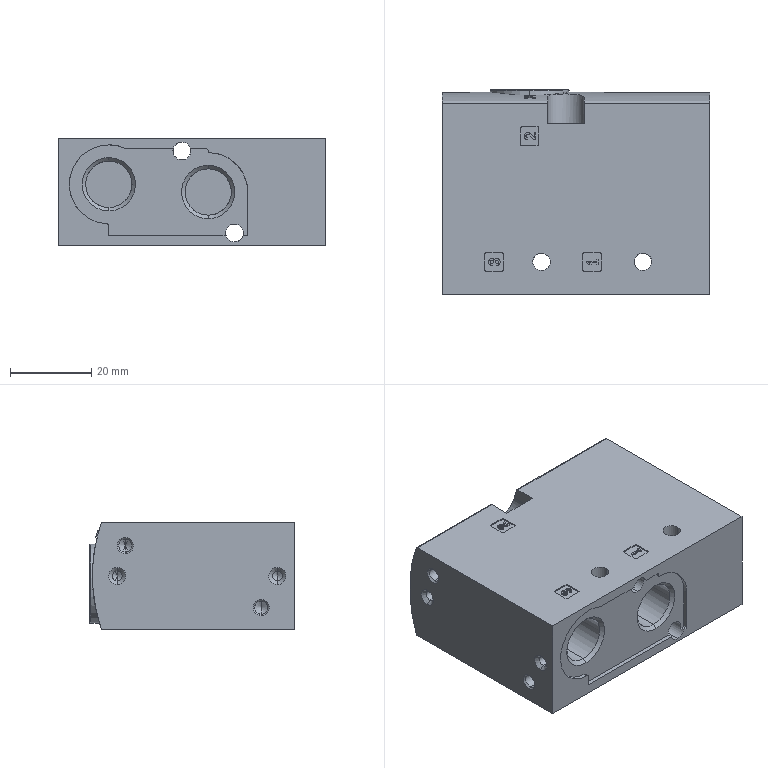Part | SolidWorks | features BaseBody 1 | 1 solid | 225 faces | box 66 x 50.5 x 26.5 mm | volume 77595 mm3 | plane 112 | cylinder 85 | cone 26 | torus 2 | commonest cylinder face diameters 0.4 x27 0.912 x8 1.71 x7 2.5 x6 11.445 x6 0.798 x4